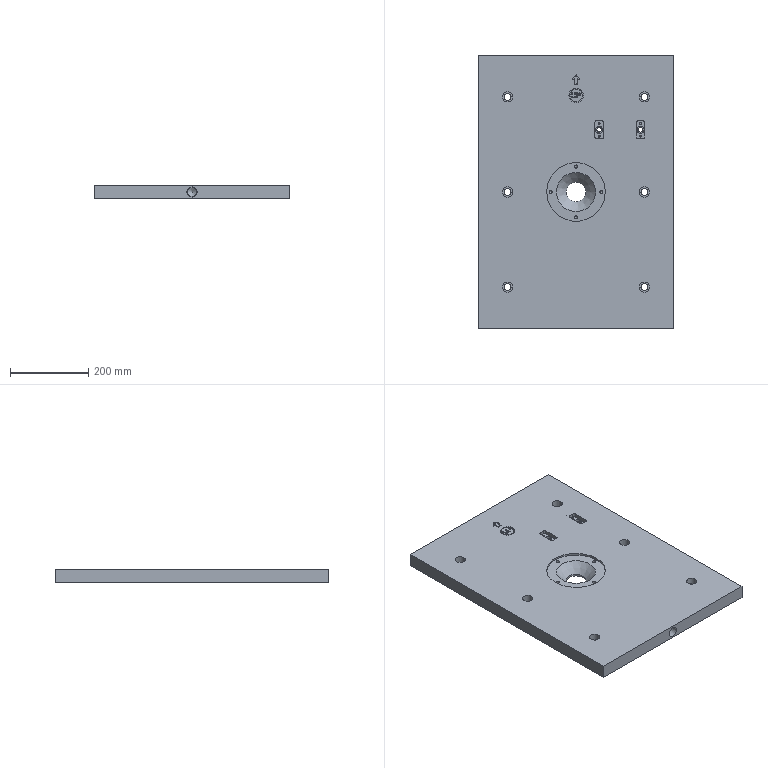Part | STEP file | AD | 1 solid | 196 faces | box 500 x 700 x 35 mm | volume 11840083 mm3 | plane 84 | cylinder 54 | spline 42 | cone 16 | commonest cylinder face diameters 4.2 x8 5 x8 8 x8 18 x8 26 x8 10 x4